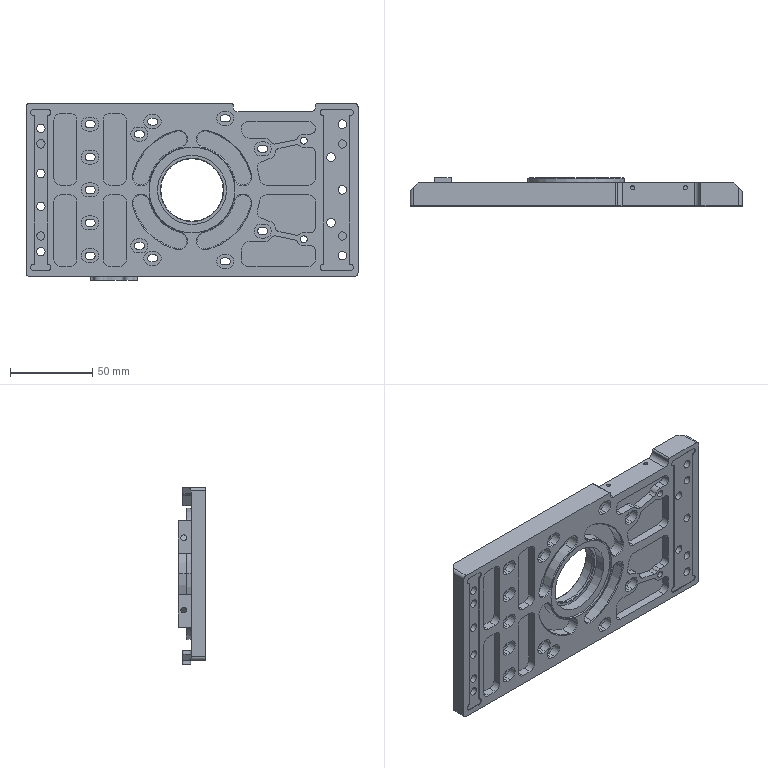Part | 1 solid | 394 faces | box 202 x 17 x 107.5 mm | volume 156437 mm3 | cylinder 196 | plane 171 | cone 26 | spline 1 | commonest cylinder face diameters 8 x36 4.2 x30 8.5 x26 5.2 x20 4 x17 6 x14